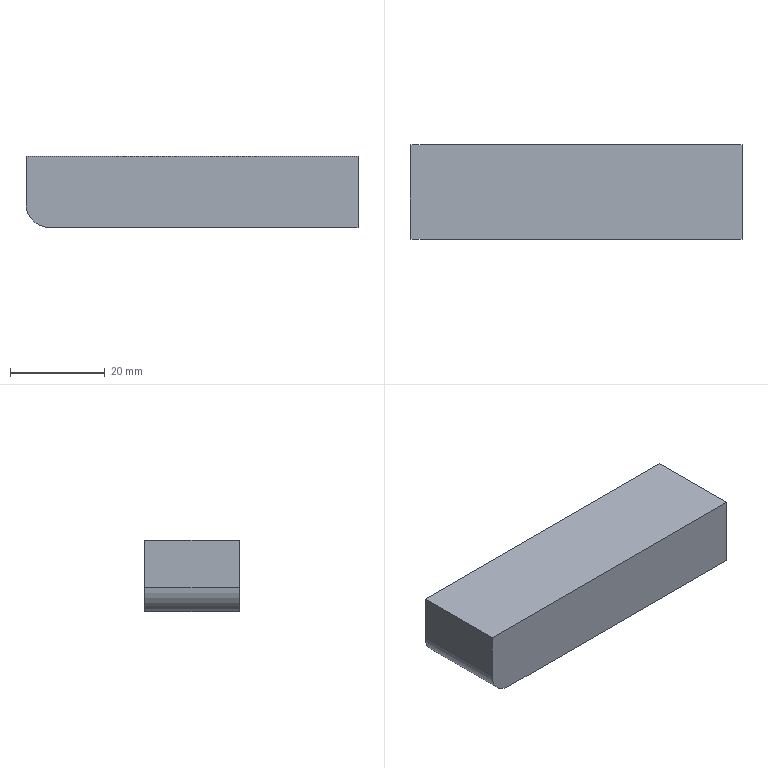Part | STEP file | 1 solid | 7 faces | box 70 x 20 x 15 mm | volume 20893 mm3 | plane 6 | cylinder 1 | commonest cylinder face diameters 10 x1
STEP:
#1=CARTESIAN_POINT('',(0.,0.,0.));
#2=DIRECTION('',(0.,0.,1.));
#3=DIRECTION('',(1.,0.,0.));
#4=AXIS2_PLACEMENT_3D('',#1,#2,#3);
#5=CARTESIAN_POINT('',(-247.863,90.5,125.451));
#6=VERTEX_POINT('',#5);
#7=CARTESIAN_POINT('',(-247.863,70.5,125.451));
#8=VERTEX_POINT('',#7);
#9=CARTESIAN_POINT('',(-247.863,69.939,125.451));
#10=DIRECTION('',(0.,-1.,0.));
#11=VECTOR('',#10,1.);
#12=LINE('',#9,#11);
#13=CARTESIAN_POINT('',(-192.81,69.939,125.451));
#14=DIRECTION('',(0.,0.,1.));
#15=DIRECTION('',(1.,0.,0.));
#16=AXIS2_PLACEMENT_3D('',#13,#14,#15);
#17=PLANE('',#16);
#18=CARTESIAN_POINT('',(-55.052,0.));
#19=DIRECTION('',(0.,-1.));
#20=VECTOR('',#19,1.);
#21=LINE('',#18,#20);
#22=(GEOMETRIC_REPRESENTATION_CONTEXT(2)PARAMETRIC_REPRESENTATION_CONTEXT()REPRESENTATION_CONTEXT('',''));
#23=DEFINITIONAL_REPRESENTATION('',(#21),#22);
#24=PCURVE('',#17,#23);
#25=CARTESIAN_POINT('',(-247.863,80.5,130.451));
#26=DIRECTION('',(0.,-1.,0.));
#27=DIRECTION('',(0.,0.,-1.));
#28=AXIS2_PLACEMENT_3D('',#25,#26,#27);
#29=CYLINDRICAL_SURFACE('',#28,5.);
#30=CARTESIAN_POINT('',(6.283,10.561));
#31=DIRECTION('',(0.,1.));
#32=VECTOR('',#31,1.);
#33=LINE('',#30,#32);
#34=(GEOMETRIC_REPRESENTATION_CONTEXT(2)PARAMETRIC_REPRESENTATION_CONTEXT()REPRESENTATION_CONTEXT('',''));
#35=DEFINITIONAL_REPRESENTATION('',(#33),#34);
#36=PCURVE('',#29,#35);
#37=SURFACE_CURVE('',#12,(#24,#36),.PCURVE_S1.);
#38=EDGE_CURVE('',#6,#8,#37,.T.);
#39=ORIENTED_EDGE('',*,*,#38,.F.);
#40=CARTESIAN_POINT('',(-182.863,90.5,125.451));
#41=VERTEX_POINT('',#40);
#42=CARTESIAN_POINT('',(-192.81,90.5,125.451));
#43=DIRECTION('',(-1.,0.,0.));
#44=VECTOR('',#43,1.);
#45=LINE('',#42,#44);
#46=CARTESIAN_POINT('',(0.,20.561));
#47=DIRECTION('',(-1.,0.));
#48=VECTOR('',#47,1.);
#49=LINE('',#46,#48);
#50=(GEOMETRIC_REPRESENTATION_CONTEXT(2)PARAMETRIC_REPRESENTATION_CONTEXT()REPRESENTATION_CONTEXT('',''));
#51=DEFINITIONAL_REPRESENTATION('',(#49),#50);
#52=PCURVE('',#17,#51);
#53=CARTESIAN_POINT('',(-192.81,90.5,125.451));
#54=DIRECTION('',(0.,1.,0.));
#55=DIRECTION('',(0.,0.,1.));
#56=AXIS2_PLACEMENT_3D('',#53,#54,#55);
#57=PLANE('',#56);
#58=CARTESIAN_POINT('',(0.,0.));
#59=DIRECTION('',(0.,-1.));
#60=VECTOR('',#59,1.);
#61=LINE('',#58,#60);
#62=(GEOMETRIC_REPRESENTATION_CONTEXT(2)PARAMETRIC_REPRESENTATION_CONTEXT()REPRESENTATION_CONTEXT('',''));
#63=DEFINITIONAL_REPRESENTATION('',(#61),#62);
#64=PCURVE('',#57,#63);
#65=SURFACE_CURVE('',#45,(#52,#64),.PCURVE_S1.);
#66=EDGE_CURVE('',#41,#6,#65,.T.);
#67=ORIENTED_EDGE('',*,*,#66,.F.);
#68=CARTESIAN_POINT('',(-182.863,70.5,125.451));
#69=VERTEX_POINT('',#68);
#70=CARTESIAN_POINT('',(-182.863,90.366,125.451));
#71=DIRECTION('',(0.,1.,0.));
#72=VECTOR('',#71,1.);
#73=LINE('',#70,#72);
#74=CARTESIAN_POINT('',(9.948,20.427));
#75=DIRECTION('',(0.,1.));
#76=VECTOR('',#75,1.);
#77=LINE('',#74,#76);
#78=(GEOMETRIC_REPRESENTATION_CONTEXT(2)PARAMETRIC_REPRESENTATION_CONTEXT()REPRESENTATION_CONTEXT('',''));
#79=DEFINITIONAL_REPRESENTATION('',(#77),#78);
#80=PCURVE('',#17,#79);
#81=CARTESIAN_POINT('',(-182.863,90.366,125.451));
#82=DIRECTION('',(1.,0.,0.));
#83=DIRECTION('',(0.,0.,-1.));
#84=AXIS2_PLACEMENT_3D('',#81,#82,#83);
#85=PLANE('',#84);
#86=CARTESIAN_POINT('',(0.,0.));
#87=DIRECTION('',(0.,1.));
#88=VECTOR('',#87,1.);
#89=LINE('',#86,#88);
#90=(GEOMETRIC_REPRESENTATION_CONTEXT(2)PARAMETRIC_REPRESENTATION_CONTEXT()REPRESENTATION_CONTEXT('',''));
#91=DEFINITIONAL_REPRESENTATION('',(#89),#90);
#92=PCURVE('',#85,#91);
#93=SURFACE_CURVE('',#73,(#80,#92),.PCURVE_S1.);
#94=EDGE_CURVE('',#69,#41,#93,.T.);
#95=ORIENTED_EDGE('',*,*,#94,.F.);
#96=CARTESIAN_POINT('',(-72.862,70.5,125.451));
#97=DIRECTION('',(1.,0.,0.));
#98=VECTOR('',#97,1.);
#99=LINE('',#96,#98);
#100=CARTESIAN_POINT('',(119.948,0.561));
#101=DIRECTION('',(1.,0.));
#102=VECTOR('',#101,1.);
#103=LINE('',#100,#102);
#104=(GEOMETRIC_REPRESENTATION_CONTEXT(2)PARAMETRIC_REPRESENTATION_CONTEXT()REPRESENTATION_CONTEXT('',''));
#105=DEFINITIONAL_REPRESENTATION('',(#103),#104);
#106=PCURVE('',#17,#105);
#107=CARTESIAN_POINT('',(-72.862,70.5,125.451));
#108=DIRECTION('',(0.,-1.,0.));
#109=DIRECTION('',(0.,0.,-1.));
#110=AXIS2_PLACEMENT_3D('',#107,#108,#109);
#111=PLANE('',#110);
#112=CARTESIAN_POINT('',(0.,0.));
#113=DIRECTION('',(0.,1.));
#114=VECTOR('',#113,1.);
#115=LINE('',#112,#114);
#116=(GEOMETRIC_REPRESENTATION_CONTEXT(2)PARAMETRIC_REPRESENTATION_CONTEXT()REPRESENTATION_CONTEXT('',''));
#117=DEFINITIONAL_REPRESENTATION('',(#115),#116);
#118=PCURVE('',#111,#117);
#119=SURFACE_CURVE('',#99,(#106,#118),.PCURVE_S1.);
#120=EDGE_CURVE('',#8,#69,#119,.T.);
#121=ORIENTED_EDGE('',*,*,#120,.F.);
#122=EDGE_LOOP('',(#39,#67,#95,#121));
#123=FACE_BOUND('',#122,.T.);
#124=ADVANCED_FACE('',(#123),#17,.F.);
#125=CARTESIAN_POINT('',(-252.863,70.5,130.451));
#126=VERTEX_POINT('',#125);
#127=CARTESIAN_POINT('',(-252.863,90.5,130.451));
#128=VERTEX_POINT('',#127);
#129=CARTESIAN_POINT('',(-252.863,80.5,130.451));
#130=DIRECTION('',(0.,1.,0.));
#131=VECTOR('',#130,1.);
#132=LINE('',#129,#131);
#133=CARTESIAN_POINT('',(-252.863,80.5,132.951));
#134=DIRECTION('',(1.,0.,0.));
#135=DIRECTION('',(0.,0.,-1.));
#136=AXIS2_PLACEMENT_3D('',#133,#134,#135);
#137=PLANE('',#136);
#138=CARTESIAN_POINT('',(2.5,0.));
#139=DIRECTION('',(0.,1.));
#140=VECTOR('',#139,1.);
#141=LINE('',#138,#140);
#142=(GEOMETRIC_REPRESENTATION_CONTEXT(2)PARAMETRIC_REPRESENTATION_CONTEXT()REPRESENTATION_CONTEXT('',''));
#143=DEFINITIONAL_REPRESENTATION('',(#141),#142);
#144=PCURVE('',#137,#143);
#145=CARTESIAN_POINT('',(4.712,0.));
#146=DIRECTION('',(0.,-1.));
#147=VECTOR('',#146,1.);
#148=LINE('',#145,#147);
#149=(GEOMETRIC_REPRESENTATION_CONTEXT(2)PARAMETRIC_REPRESENTATION_CONTEXT()REPRESENTATION_CONTEXT('',''));
#150=DEFINITIONAL_REPRESENTATION('',(#148),#149);
#151=PCURVE('',#29,#150);
#152=SURFACE_CURVE('',#132,(#144,#151),.PCURVE_S1.);
#153=EDGE_CURVE('',#126,#128,#152,.T.);
#154=ORIENTED_EDGE('',*,*,#153,.F.);
#155=CARTESIAN_POINT('',(-252.863,70.5,140.451));
#156=VERTEX_POINT('',#155);
#157=CARTESIAN_POINT('',(-252.863,70.5,125.451));
#158=DIRECTION('',(0.,0.,1.));
#159=VECTOR('',#158,1.);
#160=LINE('',#157,#159);
#161=CARTESIAN_POINT('',(7.5,-10.));
#162=DIRECTION('',(-1.,0.));
#163=VECTOR('',#162,1.);
#164=LINE('',#161,#163);
#165=(GEOMETRIC_REPRESENTATION_CONTEXT(2)PARAMETRIC_REPRESENTATION_CONTEXT()REPRESENTATION_CONTEXT('',''));
#166=DEFINITIONAL_REPRESENTATION('',(#164),#165);
#167=PCURVE('',#137,#166);
#168=CARTESIAN_POINT('',(0.,-180.));
#169=DIRECTION('',(-1.,0.));
#170=VECTOR('',#169,1.);
#171=LINE('',#168,#170);
#172=(GEOMETRIC_REPRESENTATION_CONTEXT(2)PARAMETRIC_REPRESENTATION_CONTEXT()REPRESENTATION_CONTEXT('',''));
#173=DEFINITIONAL_REPRESENTATION('',(#171),#172);
#174=PCURVE('',#111,#173);
#175=SURFACE_CURVE('',#160,(#167,#174),.PCURVE_S1.);
#176=EDGE_CURVE('',#126,#156,#175,.T.);
#177=ORIENTED_EDGE('',*,*,#176,.T.);
#178=CARTESIAN_POINT('',(-252.863,90.5,140.451));
#179=VERTEX_POINT('',#178);
#180=CARTESIAN_POINT('',(-252.863,69.939,140.451));
#181=DIRECTION('',(0.,1.,0.));
#182=VECTOR('',#181,1.);
#183=LINE('',#180,#182);
#184=CARTESIAN_POINT('',(-7.5,-10.561));
#185=DIRECTION('',(0.,1.));
#186=VECTOR('',#185,1.);
#187=LINE('',#184,#186);
#188=(GEOMETRIC_REPRESENTATION_CONTEXT(2)PARAMETRIC_REPRESENTATION_CONTEXT()REPRESENTATION_CONTEXT('',''));
#189=DEFINITIONAL_REPRESENTATION('',(#187),#188);
#190=PCURVE('',#137,#189);
#191=CARTESIAN_POINT('',(-192.81,69.939,140.451));
#192=DIRECTION('',(0.,0.,1.));
#193=DIRECTION('',(1.,0.,0.));
#194=AXIS2_PLACEMENT_3D('',#191,#192,#193);
#195=PLANE('',#194);
#196=CARTESIAN_POINT('',(-60.052,0.));
#197=DIRECTION('',(0.,1.));
#198=VECTOR('',#197,1.);
#199=LINE('',#196,#198);
#200=(GEOMETRIC_REPRESENTATION_CONTEXT(2)PARAMETRIC_REPRESENTATION_CONTEXT()REPRESENTATION_CONTEXT('',''));
#201=DEFINITIONAL_REPRESENTATION('',(#199),#200);
#202=PCURVE('',#195,#201);
#203=SURFACE_CURVE('',#183,(#190,#202),.PCURVE_S1.);
#204=EDGE_CURVE('',#156,#179,#203,.T.);
#205=ORIENTED_EDGE('',*,*,#204,.T.);
#206=CARTESIAN_POINT('',(-252.863,90.5,125.451));
#207=DIRECTION('',(0.,0.,-1.));
#208=VECTOR('',#207,1.);
#209=LINE('',#206,#208);
#210=CARTESIAN_POINT('',(7.5,10.));
#211=DIRECTION('',(1.,0.));
#212=VECTOR('',#211,1.);
#213=LINE('',#210,#212);
#214=(GEOMETRIC_REPRESENTATION_CONTEXT(2)PARAMETRIC_REPRESENTATION_CONTEXT()REPRESENTATION_CONTEXT('',''));
#215=DEFINITIONAL_REPRESENTATION('',(#213),#214);
#216=PCURVE('',#137,#215);
#217=CARTESIAN_POINT('',(0.,-60.052));
#218=DIRECTION('',(-1.,0.));
#219=VECTOR('',#218,1.);
#220=LINE('',#217,#219);
#221=(GEOMETRIC_REPRESENTATION_CONTEXT(2)PARAMETRIC_REPRESENTATION_CONTEXT()REPRESENTATION_CONTEXT('',''));
#222=DEFINITIONAL_REPRESENTATION('',(#220),#221);
#223=PCURVE('',#57,#222);
#224=SURFACE_CURVE('',#209,(#216,#223),.PCURVE_S1.);
#225=EDGE_CURVE('',#179,#128,#224,.T.);
#226=ORIENTED_EDGE('',*,*,#225,.T.);
#227=EDGE_LOOP('',(#154,#177,#205,#226));
#228=FACE_BOUND('',#227,.T.);
#229=ADVANCED_FACE('',(#228),#137,.F.);
#230=CARTESIAN_POINT('',(-247.863,70.5,130.451));
#231=DIRECTION('',(0.,1.,0.));
#232=DIRECTION('',(0.,0.,1.));
#233=AXIS2_PLACEMENT_3D('',#230,#231,#232);
#234=CIRCLE('',#233,5.);
#235=CARTESIAN_POINT('',(-10.,-175.));
#236=CARTESIAN_POINT('',(-10.,-166.34));
#237=CARTESIAN_POINT('',(-2.5,-170.67));
#238=CARTESIAN_POINT('',(5.,-175.));
#239=CARTESIAN_POINT('',(-2.5,-179.33));
#240=CARTESIAN_POINT('',(-10.,-183.66));
#241=CARTESIAN_POINT('',(-10.,-175.));
#242=(BOUNDED_CURVE()B_SPLINE_CURVE(2,(#235,#236,#237,#238,#239,#240,#241),.UNSPECIFIED.,.T.,.F.)B_SPLINE_CURVE_WITH_KNOTS((1,2,2,2,2,1),(-2.094,0.,2.094,4.189,6.283,8.378),.UNSPECIFIED.)CURVE()GEOMETRIC_REPRESENTATION_ITEM()RATIONAL_B_SPLINE_CURVE((1.,0.5,1.,0.5,1.,0.5,1.))REPRESENTATION_ITEM(''));
#243=(GEOMETRIC_REPRESENTATION_CONTEXT(2)PARAMETRIC_REPRESENTATION_CONTEXT()REPRESENTATION_CONTEXT('',''));
#244=DEFINITIONAL_REPRESENTATION('',(#242),#243);
#245=PCURVE('',#111,#244);
#246=CARTESIAN_POINT('',(9.425,10.));
#247=DIRECTION('',(-1.,0.));
#248=VECTOR('',#247,1.);
#249=LINE('',#246,#248);
#250=(GEOMETRIC_REPRESENTATION_CONTEXT(2)PARAMETRIC_REPRESENTATION_CONTEXT()REPRESENTATION_CONTEXT('',''));
#251=DEFINITIONAL_REPRESENTATION('',(#249),#250);
#252=PCURVE('',#29,#251);
#253=SURFACE_CURVE('',#234,(#245,#252),.PCURVE_S1.);
#254=EDGE_CURVE('',#8,#126,#253,.T.);
#255=ORIENTED_EDGE('',*,*,#254,.F.);
#256=ORIENTED_EDGE('',*,*,#120,.T.);
#257=CARTESIAN_POINT('',(-182.863,70.5,140.451));
#258=VERTEX_POINT('',#257);
#259=CARTESIAN_POINT('',(-182.863,70.5,125.451));
#260=DIRECTION('',(0.,0.,1.));
#261=VECTOR('',#260,1.);
#262=LINE('',#259,#261);
#263=CARTESIAN_POINT('',(0.,-110.));
#264=DIRECTION('',(-1.,0.));
#265=VECTOR('',#264,1.);
#266=LINE('',#263,#265);
#267=(GEOMETRIC_REPRESENTATION_CONTEXT(2)PARAMETRIC_REPRESENTATION_CONTEXT()REPRESENTATION_CONTEXT('',''));
#268=DEFINITIONAL_REPRESENTATION('',(#266),#267);
#269=PCURVE('',#111,#268);
#270=CARTESIAN_POINT('',(0.,-19.866));
#271=DIRECTION('',(-1.,0.));
#272=VECTOR('',#271,1.);
#273=LINE('',#270,#272);
#274=(GEOMETRIC_REPRESENTATION_CONTEXT(2)PARAMETRIC_REPRESENTATION_CONTEXT()REPRESENTATION_CONTEXT('',''));
#275=DEFINITIONAL_REPRESENTATION('',(#273),#274);
#276=PCURVE('',#85,#275);
#277=SURFACE_CURVE('',#262,(#269,#276),.PCURVE_S1.);
#278=EDGE_CURVE('',#69,#258,#277,.T.);
#279=ORIENTED_EDGE('',*,*,#278,.T.);
#280=CARTESIAN_POINT('',(-72.862,70.5,140.451));
#281=DIRECTION('',(1.,0.,0.));
#282=VECTOR('',#281,1.);
#283=LINE('',#280,#282);
#284=CARTESIAN_POINT('',(-15.,0.));
#285=DIRECTION('',(0.,1.));
#286=VECTOR('',#285,1.);
#287=LINE('',#284,#286);
#288=(GEOMETRIC_REPRESENTATION_CONTEXT(2)PARAMETRIC_REPRESENTATION_CONTEXT()REPRESENTATION_CONTEXT('',''));
#289=DEFINITIONAL_REPRESENTATION('',(#287),#288);
#290=PCURVE('',#111,#289);
#291=CARTESIAN_POINT('',(119.948,0.561));
#292=DIRECTION('',(1.,0.));
#293=VECTOR('',#292,1.);
#294=LINE('',#291,#293);
#295=(GEOMETRIC_REPRESENTATION_CONTEXT(2)PARAMETRIC_REPRESENTATION_CONTEXT()REPRESENTATION_CONTEXT('',''));
#296=DEFINITIONAL_REPRESENTATION('',(#294),#295);
#297=PCURVE('',#195,#296);
#298=SURFACE_CURVE('',#283,(#290,#297),.PCURVE_S1.);
#299=EDGE_CURVE('',#156,#258,#298,.T.);
#300=ORIENTED_EDGE('',*,*,#299,.F.);
#301=ORIENTED_EDGE('',*,*,#176,.F.);
#302=EDGE_LOOP('',(#255,#256,#279,#300,#301));
#303=FACE_BOUND('',#302,.T.);
#304=ADVANCED_FACE('',(#303),#111,.T.);
#305=CARTESIAN_POINT('',(-182.863,90.5,140.451));
#306=VERTEX_POINT('',#305);
#307=CARTESIAN_POINT('',(-182.863,90.366,140.451));
#308=DIRECTION('',(0.,1.,0.));
#309=VECTOR('',#308,1.);
#310=LINE('',#307,#309);
#311=CARTESIAN_POINT('',(-15.,0.));
#312=DIRECTION('',(0.,1.));
#313=VECTOR('',#312,1.);
#314=LINE('',#311,#313);
#315=(GEOMETRIC_REPRESENTATION_CONTEXT(2)PARAMETRIC_REPRESENTATION_CONTEXT()REPRESENTATION_CONTEXT('',''));
#316=DEFINITIONAL_REPRESENTATION('',(#314),#315);
#317=PCURVE('',#85,#316);
#318=CARTESIAN_POINT('',(9.948,20.427));
#319=DIRECTION('',(0.,1.));
#320=VECTOR('',#319,1.);
#321=LINE('',#318,#320);
#322=(GEOMETRIC_REPRESENTATION_CONTEXT(2)PARAMETRIC_REPRESENTATION_CONTEXT()REPRESENTATION_CONTEXT('',''));
#323=DEFINITIONAL_REPRESENTATION('',(#321),#322);
#324=PCURVE('',#195,#323);
#325=SURFACE_CURVE('',#310,(#317,#324),.PCURVE_S1.);
#326=EDGE_CURVE('',#258,#306,#325,.T.);
#327=ORIENTED_EDGE('',*,*,#326,.F.);
#328=ORIENTED_EDGE('',*,*,#278,.F.);
#329=ORIENTED_EDGE('',*,*,#94,.T.);
#330=CARTESIAN_POINT('',(-182.863,90.5,136.951));
#331=VERTEX_POINT('',#330);
#332=CARTESIAN_POINT('',(-182.863,90.5,125.451));
#333=DIRECTION('',(0.,0.,1.));
#334=VECTOR('',#333,1.);
#335=LINE('',#332,#334);
#336=CARTESIAN_POINT('',(0.,0.134));
#337=DIRECTION('',(-1.,0.));
#338=VECTOR('',#337,1.);
#339=LINE('',#336,#338);
#340=(GEOMETRIC_REPRESENTATION_CONTEXT(2)PARAMETRIC_REPRESENTATION_CONTEXT()REPRESENTATION_CONTEXT('',''));
#341=DEFINITIONAL_REPRESENTATION('',(#339),#340);
#342=PCURVE('',#85,#341);
#343=CARTESIAN_POINT('',(0.,9.948));
#344=DIRECTION('',(1.,0.));
#345=VECTOR('',#344,1.);
#346=LINE('',#343,#345);
#347=(GEOMETRIC_REPRESENTATION_CONTEXT(2)PARAMETRIC_REPRESENTATION_CONTEXT()REPRESENTATION_CONTEXT('',''));
#348=DEFINITIONAL_REPRESENTATION('',(#346),#347);
#349=PCURVE('',#57,#348);
#350=SURFACE_CURVE('',#335,(#342,#349),.PCURVE_S1.);
#351=EDGE_CURVE('',#41,#331,#350,.T.);
#352=ORIENTED_EDGE('',*,*,#351,.T.);
#353=CARTESIAN_POINT('',(-182.863,90.5,136.951));
#354=CARTESIAN_POINT('',(-182.863,90.5,138.118));
#355=CARTESIAN_POINT('',(-182.863,90.5,139.285));
#356=CARTESIAN_POINT('',(-182.863,90.5,140.451));
#357=B_SPLINE_CURVE_WITH_KNOTS('',3,(#353,#354,#355,#356),.UNSPECIFIED.,.F.,.F.,(4,4),(0.7667,1.),.PIECEWISE_BEZIER_KNOTS.);
#358=CARTESIAN_POINT('',(-11.5,0.134));
#359=CARTESIAN_POINT('',(-12.667,0.134));
#360=CARTESIAN_POINT('',(-13.833,0.134));
#361=CARTESIAN_POINT('',(-15.,0.134));
#362=B_SPLINE_CURVE_WITH_KNOTS('',3,(#358,#359,#360,#361),.UNSPECIFIED.,.F.,.F.,(4,4),(0.7667,1.),.PIECEWISE_BEZIER_KNOTS.);
#363=(GEOMETRIC_REPRESENTATION_CONTEXT(2)PARAMETRIC_REPRESENTATION_CONTEXT()REPRESENTATION_CONTEXT('',''));
#364=DEFINITIONAL_REPRESENTATION('',(#362),#363);
#365=PCURVE('',#85,#364);
#366=CARTESIAN_POINT('',(11.5,9.948));
#367=CARTESIAN_POINT('',(12.667,9.948));
#368=CARTESIAN_POINT('',(13.833,9.948));
#369=CARTESIAN_POINT('',(15.,9.948));
#370=B_SPLINE_CURVE_WITH_KNOTS('',3,(#366,#367,#368,#369),.UNSPECIFIED.,.F.,.F.,(4,4),(0.7667,1.),.PIECEWISE_BEZIER_KNOTS.);
#371=(GEOMETRIC_REPRESENTATION_CONTEXT(2)PARAMETRIC_REPRESENTATION_CONTEXT()REPRESENTATION_CONTEXT('',''));
#372=DEFINITIONAL_REPRESENTATION('',(#370),#371);
#373=PCURVE('',#57,#372);
#374=SURFACE_CURVE('',#357,(#365,#373),.PCURVE_S1.);
#375=EDGE_CURVE('',#331,#306,#374,.T.);
#376=ORIENTED_EDGE('',*,*,#375,.T.);
#377=EDGE_LOOP('',(#327,#328,#329,#352,#376));
#378=FACE_BOUND('',#377,.T.);
#379=ADVANCED_FACE('',(#378),#85,.T.);
#380=CARTESIAN_POINT('',(-247.863,90.5,130.451));
#381=DIRECTION('',(0.,-1.,0.));
#382=DIRECTION('',(0.,0.,1.));
#383=AXIS2_PLACEMENT_3D('',#380,#381,#382);
#384=CIRCLE('',#383,5.);
#385=CARTESIAN_POINT('',(10.,-55.052));
#386=CARTESIAN_POINT('',(10.,-63.712));
#387=CARTESIAN_POINT('',(2.5,-59.382));
#388=CARTESIAN_POINT('',(-5.,-55.052));
#389=CARTESIAN_POINT('',(2.5,-50.722));
#390=CARTESIAN_POINT('',(10.,-46.392));
#391=CARTESIAN_POINT('',(10.,-55.052));
#392=(BOUNDED_CURVE()B_SPLINE_CURVE(2,(#385,#386,#387,#388,#389,#390,#391),.UNSPECIFIED.,.T.,.F.)B_SPLINE_CURVE_WITH_KNOTS((1,2,2,2,2,1),(-2.094,0.,2.094,4.189,6.283,8.378),.UNSPECIFIED.)CURVE()GEOMETRIC_REPRESENTATION_ITEM()RATIONAL_B_SPLINE_CURVE((1.,0.5,1.,0.5,1.,0.5,1.))REPRESENTATION_ITEM(''));
#393=(GEOMETRIC_REPRESENTATION_CONTEXT(2)PARAMETRIC_REPRESENTATION_CONTEXT()REPRESENTATION_CONTEXT('',''));
#394=DEFINITIONAL_REPRESENTATION('',(#392),#393);
#395=PCURVE('',#57,#394);
#396=CARTESIAN_POINT('',(3.142,-10.));
#397=DIRECTION('',(1.,0.));
#398=VECTOR('',#397,1.);
#399=LINE('',#396,#398);
#400=(GEOMETRIC_REPRESENTATION_CONTEXT(2)PARAMETRIC_REPRESENTATION_CONTEXT()REPRESENTATION_CONTEXT('',''));
#401=DEFINITIONAL_REPRESENTATION('',(#399),#400);
#402=PCURVE('',#29,#401);
#403=SURFACE_CURVE('',#384,(#395,#402),.PCURVE_S1.);
#404=EDGE_CURVE('',#128,#6,#403,.T.);
#405=ORIENTED_EDGE('',*,*,#404,.F.);
#406=ORIENTED_EDGE('',*,*,#225,.F.);
#407=CARTESIAN_POINT('',(-192.81,90.5,140.451));
#408=DIRECTION('',(-1.,0.,0.));
#409=VECTOR('',#408,1.);
#410=LINE('',#407,#409);
#411=CARTESIAN_POINT('',(15.,0.));
#412=DIRECTION('',(0.,-1.));
#413=VECTOR('',#412,1.);
#414=LINE('',#411,#413);
#415=(GEOMETRIC_REPRESENTATION_CONTEXT(2)PARAMETRIC_REPRESENTATION_CONTEXT()REPRESENTATION_CONTEXT('',''));
#416=DEFINITIONAL_REPRESENTATION('',(#414),#415);
#417=PCURVE('',#57,#416);
#418=CARTESIAN_POINT('',(0.,20.561));
#419=DIRECTION('',(-1.,0.));
#420=VECTOR('',#419,1.);
#421=LINE('',#418,#420);
#422=(GEOMETRIC_REPRESENTATION_CONTEXT(2)PARAMETRIC_REPRESENTATION_CONTEXT()REPRESENTATION_CONTEXT('',''));
#423=DEFINITIONAL_REPRESENTATION('',(#421),#422);
#424=PCURVE('',#195,#423);
#425=SURFACE_CURVE('',#410,(#417,#424),.PCURVE_S1.);
#426=EDGE_CURVE('',#306,#179,#425,.T.);
#427=ORIENTED_EDGE('',*,*,#426,.F.);
#428=ORIENTED_EDGE('',*,*,#375,.F.);
#429=ORIENTED_EDGE('',*,*,#351,.F.);
#430=ORIENTED_EDGE('',*,*,#66,.T.);
#431=EDGE_LOOP('',(#405,#406,#427,#428,#429,#430));
#432=FACE_BOUND('',#431,.T.);
#433=ADVANCED_FACE('',(#432),#57,.T.);
#434=ORIENTED_EDGE('',*,*,#204,.F.);
#435=ORIENTED_EDGE('',*,*,#299,.T.);
#436=ORIENTED_EDGE('',*,*,#326,.T.);
#437=ORIENTED_EDGE('',*,*,#426,.T.);
#438=EDGE_LOOP('',(#434,#435,#436,#437));
#439=FACE_BOUND('',#438,.T.);
#440=ADVANCED_FACE('',(#439),#195,.T.);
#441=ORIENTED_EDGE('',*,*,#254,.T.);
#442=ORIENTED_EDGE('',*,*,#153,.T.);
#443=ORIENTED_EDGE('',*,*,#404,.T.);
#444=ORIENTED_EDGE('',*,*,#38,.T.);
#445=EDGE_LOOP('',(#441,#442,#443,#444));
#446=FACE_BOUND('',#445,.T.);
#447=ADVANCED_FACE('',(#446),#29,.T.);
#448=CLOSED_SHELL('',(#124,#229,#304,#379,#433,#440,#447));
#449=MANIFOLD_SOLID_BREP('',#448);
#450=(LENGTH_UNIT()NAMED_UNIT(*)SI_UNIT(.MILLI.,.METRE.));
#451=UNCERTAINTY_MEASURE_WITH_UNIT(LENGTH_MEASURE(0.0000001),#450,'','');
#452=(NAMED_UNIT(*)PLANE_ANGLE_UNIT()SI_UNIT($,.RADIAN.));
#453=(NAMED_UNIT(*)SI_UNIT($,.STERADIAN.)SOLID_ANGLE_UNIT());
#454=(GEOMETRIC_REPRESENTATION_CONTEXT(3)GLOBAL_UNCERTAINTY_ASSIGNED_CONTEXT((#451))GLOBAL_UNIT_ASSIGNED_CONTEXT((#450,#452,#453))REPRESENTATION_CONTEXT('',''));
#455=ADVANCED_BREP_SHAPE_REPRESENTATION('',(#4,#449),#454);